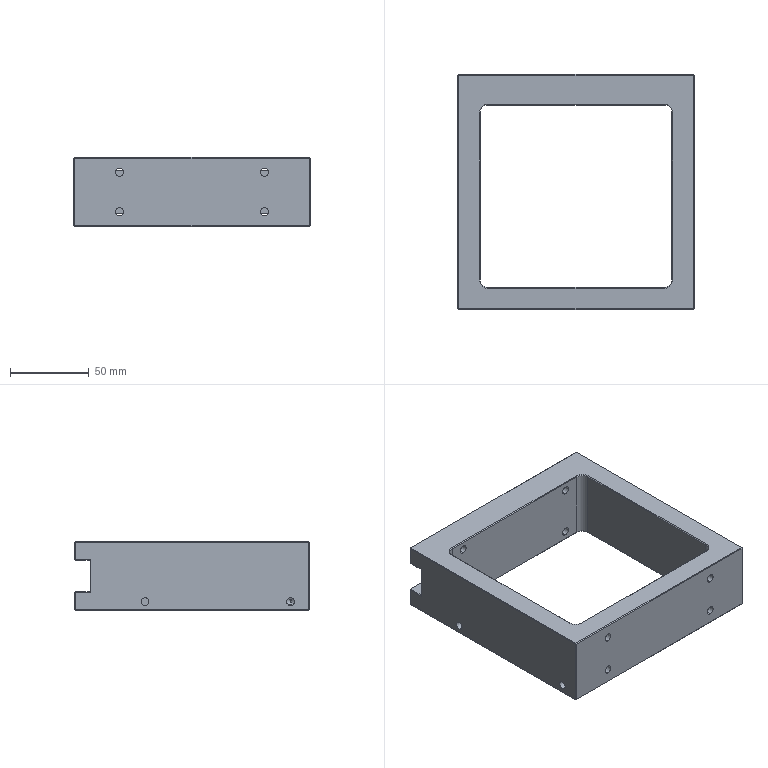Part | NX | features BREP 1 | 1 solid | 98 faces | box 150 x 149.38 x 44 mm | volume 330410 mm3 | plane 56 | cylinder 24 | cone 18 | commonest cylinder face diameters 5.2 x16 5 x4 10 x4